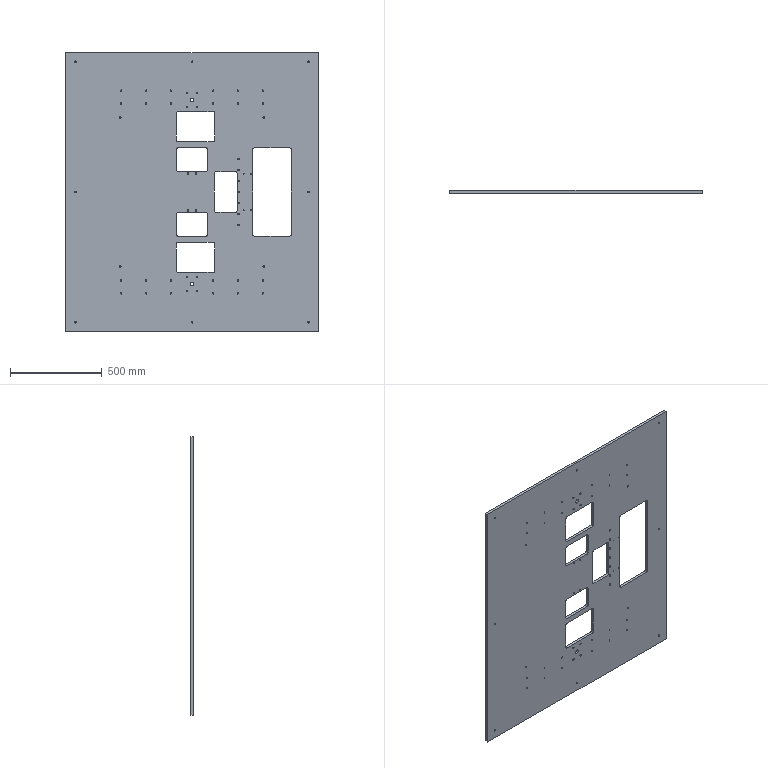Part | STEP file | 0244_201_Plate | 1 solid | 176 faces | box 1375 x 15 x 1515 mm | volume 27581245 mm3 | cylinder 146 | plane 30 | commonest cylinder face diameters 6.8 x56 9 x46 20 x28 5.5 x8 8.5 x8